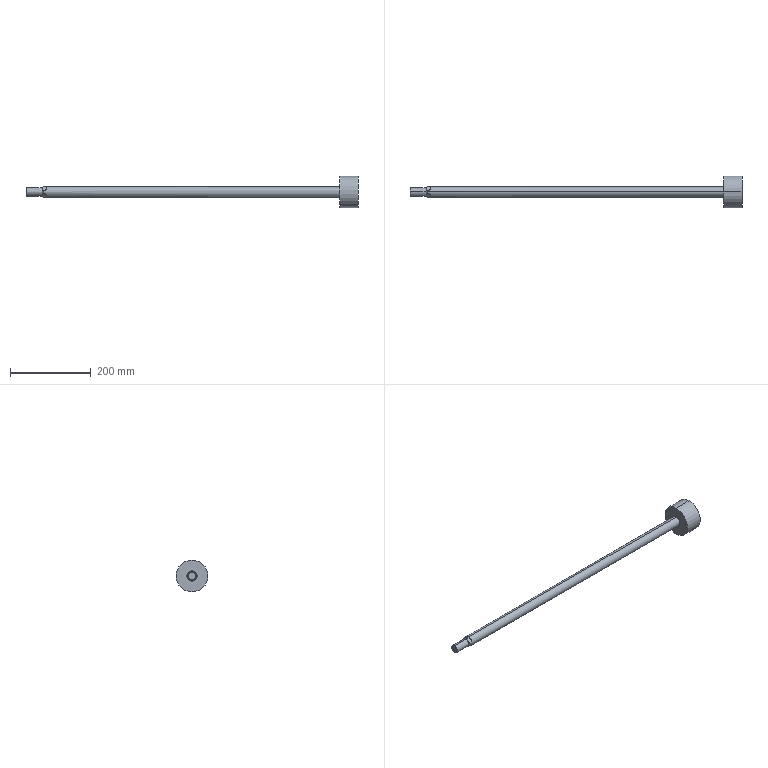Part | NX | features BREP 1 | 1 solid | 21 faces | box 822.5 x 78.6 x 78.6 mm | volume 592313 mm3 | plane 11 | cylinder 6 | cone 4 | commonest cylinder face diameters 20 x2 25 x2 78.6 x2
STEP:
#1=CARTESIAN_POINT('',(691.5,0.,12.5));
#2=VERTEX_POINT('',#1);
#3=CARTESIAN_POINT('',(691.5,0.,-12.5));
#4=VERTEX_POINT('',#3);
#5=CARTESIAN_POINT('',(691.5,0.,0.));
#6=DIRECTION('',(-1.,0.,0.));
#7=DIRECTION('',(0.,0.,1.));
#8=AXIS2_PLACEMENT_3D('',#5,#6,#7);
#9=CIRCLE('',#8,12.5);
#10=EDGE_CURVE('',#2,#4,#9,.T.);
#11=ORIENTED_EDGE('',*,*,#10,.T.);
#12=CARTESIAN_POINT('',(-43.5,0.,-12.5));
#13=VERTEX_POINT('',#12);
#14=CARTESIAN_POINT('',(736.5,0.,-12.5));
#15=DIRECTION('',(-1.,0.,0.));
#16=VECTOR('',#15,1000.);
#17=LINE('',#14,#16);
#18=EDGE_CURVE('',#13,#4,#17,.F.);
#19=ORIENTED_EDGE('',*,*,#18,.F.);
#20=CARTESIAN_POINT('',(-43.5,3.58,-11.976));
#21=VERTEX_POINT('',#20);
#22=CARTESIAN_POINT('',(-43.5,0.,0.));
#23=DIRECTION('',(1.,0.,0.));
#24=DIRECTION('',(0.,0.,1.));
#25=AXIS2_PLACEMENT_3D('',#22,#23,#24);
#26=CIRCLE('',#25,12.5);
#27=EDGE_CURVE('',#13,#21,#26,.T.);
#28=ORIENTED_EDGE('',*,*,#27,.T.);
#29=CARTESIAN_POINT('',(-37.1,3.58,-11.976));
#30=VERTEX_POINT('',#29);
#31=CARTESIAN_POINT('',(736.5,3.58,-11.976));
#32=DIRECTION('',(1.,0.,0.));
#33=VECTOR('',#32,1000.);
#34=LINE('',#31,#33);
#35=EDGE_CURVE('',#21,#30,#34,.T.);
#36=ORIENTED_EDGE('',*,*,#35,.T.);
#37=CARTESIAN_POINT('',(-37.1,11.976,-3.58));
#38=VERTEX_POINT('',#37);
#39=CARTESIAN_POINT('',(-37.1,3.58,-11.976));
#40=CARTESIAN_POINT('',(-35.057,7.702,-10.744));
#41=CARTESIAN_POINT('',(-35.057,10.744,-7.702));
#42=CARTESIAN_POINT('',(-37.1,11.976,-3.58));
#43=(BOUNDED_CURVE()B_SPLINE_CURVE(3,(#39,#40,#41,#42),.UNSPECIFIED.,.F.,.F.)B_SPLINE_CURVE_WITH_KNOTS((4,4),(2.647,3.637),.UNSPECIFIED.)CURVE()GEOMETRIC_REPRESENTATION_ITEM()RATIONAL_B_SPLINE_CURVE((1.,0.92,0.92,1.))REPRESENTATION_ITEM(''));
#44=EDGE_CURVE('',#30,#38,#43,.T.);
#45=ORIENTED_EDGE('',*,*,#44,.T.);
#46=CARTESIAN_POINT('',(-43.5,11.976,-3.58));
#47=VERTEX_POINT('',#46);
#48=CARTESIAN_POINT('',(736.5,11.976,-3.58));
#49=DIRECTION('',(-1.,0.,0.));
#50=VECTOR('',#49,1000.);
#51=LINE('',#48,#50);
#52=EDGE_CURVE('',#38,#47,#51,.T.);
#53=ORIENTED_EDGE('',*,*,#52,.T.);
#54=CARTESIAN_POINT('',(-43.5,11.976,3.58));
#55=VERTEX_POINT('',#54);
#56=CARTESIAN_POINT('',(-43.5,0.,0.));
#57=DIRECTION('',(1.,0.,0.));
#58=DIRECTION('',(0.,0.,1.));
#59=AXIS2_PLACEMENT_3D('',#56,#57,#58);
#60=CIRCLE('',#59,12.5);
#61=EDGE_CURVE('',#47,#55,#60,.T.);
#62=ORIENTED_EDGE('',*,*,#61,.T.);
#63=CARTESIAN_POINT('',(-37.1,11.976,3.58));
#64=VERTEX_POINT('',#63);
#65=CARTESIAN_POINT('',(736.5,11.976,3.58));
#66=DIRECTION('',(1.,0.,0.));
#67=VECTOR('',#66,1000.);
#68=LINE('',#65,#67);
#69=EDGE_CURVE('',#55,#64,#68,.T.);
#70=ORIENTED_EDGE('',*,*,#69,.T.);
#71=CARTESIAN_POINT('',(-37.1,3.58,11.976));
#72=VERTEX_POINT('',#71);
#73=CARTESIAN_POINT('',(-37.1,11.976,3.58));
#74=CARTESIAN_POINT('',(-35.057,10.744,7.702));
#75=CARTESIAN_POINT('',(-35.057,7.702,10.744));
#76=CARTESIAN_POINT('',(-37.1,3.58,11.976));
#77=(BOUNDED_CURVE()B_SPLINE_CURVE(3,(#73,#74,#75,#76),.UNSPECIFIED.,.F.,.F.)B_SPLINE_CURVE_WITH_KNOTS((4,4),(2.647,3.637),.UNSPECIFIED.)CURVE()GEOMETRIC_REPRESENTATION_ITEM()RATIONAL_B_SPLINE_CURVE((1.,0.92,0.92,1.))REPRESENTATION_ITEM(''));
#78=EDGE_CURVE('',#64,#72,#77,.T.);
#79=ORIENTED_EDGE('',*,*,#78,.T.);
#80=CARTESIAN_POINT('',(-43.5,3.58,11.976));
#81=VERTEX_POINT('',#80);
#82=CARTESIAN_POINT('',(736.5,3.58,11.976));
#83=DIRECTION('',(-1.,0.,0.));
#84=VECTOR('',#83,1000.);
#85=LINE('',#82,#84);
#86=EDGE_CURVE('',#72,#81,#85,.T.);
#87=ORIENTED_EDGE('',*,*,#86,.T.);
#88=CARTESIAN_POINT('',(-43.5,0.,12.5));
#89=VERTEX_POINT('',#88);
#90=CARTESIAN_POINT('',(-43.5,0.,0.));
#91=DIRECTION('',(1.,0.,0.));
#92=DIRECTION('',(0.,0.,1.));
#93=AXIS2_PLACEMENT_3D('',#90,#91,#92);
#94=CIRCLE('',#93,12.5);
#95=EDGE_CURVE('',#81,#89,#94,.T.);
#96=ORIENTED_EDGE('',*,*,#95,.T.);
#97=CARTESIAN_POINT('',(736.5,0.,12.5));
#98=DIRECTION('',(-1.,0.,0.));
#99=VECTOR('',#98,1000.);
#100=LINE('',#97,#99);
#101=EDGE_CURVE('',#89,#2,#100,.F.);
#102=ORIENTED_EDGE('',*,*,#101,.T.);
#103=EDGE_LOOP('',(#11,#19,#28,#36,#45,#53,#62,#70,#79,#87,#96,#102));
#104=FACE_BOUND('',#103,.T.);
#105=CARTESIAN_POINT('',(736.5,0.,0.));
#106=DIRECTION('',(-1.,0.,0.));
#107=DIRECTION('',(0.,0.,1.));
#108=AXIS2_PLACEMENT_3D('',#105,#106,#107);
#109=CYLINDRICAL_SURFACE('',#108,12.5);
#110=ADVANCED_FACE('',(#104),#109,.T.);
#111=CARTESIAN_POINT('',(-46.,0.,-10.));
#112=VERTEX_POINT('',#111);
#113=CARTESIAN_POINT('',(-46.,0.,10.));
#114=VERTEX_POINT('',#113);
#115=CARTESIAN_POINT('',(-46.,0.,0.));
#116=DIRECTION('',(1.,0.,0.));
#117=DIRECTION('',(0.,0.,-1.));
#118=AXIS2_PLACEMENT_3D('',#115,#116,#117);
#119=CIRCLE('',#118,10.);
#120=EDGE_CURVE('',#112,#114,#119,.T.);
#121=ORIENTED_EDGE('',*,*,#120,.T.);
#122=CARTESIAN_POINT('',(-43.5,0.,12.5));
#123=DIRECTION('',(0.7071,0.,0.7071));
#124=VECTOR('',#123,1000.);
#125=LINE('',#122,#124);
#126=EDGE_CURVE('',#114,#89,#125,.T.);
#127=ORIENTED_EDGE('',*,*,#126,.T.);
#128=ORIENTED_EDGE('',*,*,#95,.F.);
#129=CARTESIAN_POINT('',(-43.5,11.976,3.58));
#130=CARTESIAN_POINT('',(-43.979,11.263,4.294));
#131=CARTESIAN_POINT('',(-44.505,10.309,5.247));
#132=CARTESIAN_POINT('',(-44.937,8.824,6.732));
#133=CARTESIAN_POINT('',(-45.032,7.764,7.792));
#134=CARTESIAN_POINT('',(-44.933,6.711,8.845));
#135=CARTESIAN_POINT('',(-44.598,5.578,9.979));
#136=CARTESIAN_POINT('',(-44.158,4.637,10.919));
#137=CARTESIAN_POINT('',(-43.738,3.934,11.623));
#138=CARTESIAN_POINT('',(-43.5,3.58,11.976));
#139=B_SPLINE_CURVE_WITH_KNOTS('',3,(#129,#130,#131,#132,#133,#134,#135,#136,#137,#138),.UNSPECIFIED.,.F.,.F.,(4,1,1,1,1,1,1,4),(0.,0.25,0.375,0.5,0.625,0.75,0.875,1.),.UNSPECIFIED.);
#140=EDGE_CURVE('',#81,#55,#139,.F.);
#141=ORIENTED_EDGE('',*,*,#140,.T.);
#142=ORIENTED_EDGE('',*,*,#61,.F.);
#143=CARTESIAN_POINT('',(-43.5,3.58,-11.976));
#144=CARTESIAN_POINT('',(-43.979,4.294,-11.263));
#145=CARTESIAN_POINT('',(-44.505,5.247,-10.309));
#146=CARTESIAN_POINT('',(-44.937,6.732,-8.824));
#147=CARTESIAN_POINT('',(-45.032,7.792,-7.764));
#148=CARTESIAN_POINT('',(-44.933,8.845,-6.711));
#149=CARTESIAN_POINT('',(-44.598,9.979,-5.578));
#150=CARTESIAN_POINT('',(-44.158,10.919,-4.637));
#151=CARTESIAN_POINT('',(-43.738,11.623,-3.934));
#152=CARTESIAN_POINT('',(-43.5,11.976,-3.58));
#153=B_SPLINE_CURVE_WITH_KNOTS('',3,(#143,#144,#145,#146,#147,#148,#149,#150,#151,#152),.UNSPECIFIED.,.F.,.F.,(4,1,1,1,1,1,1,4),(0.,0.25,0.375,0.5,0.625,0.75,0.875,1.),.UNSPECIFIED.);
#154=EDGE_CURVE('',#47,#21,#153,.F.);
#155=ORIENTED_EDGE('',*,*,#154,.T.);
#156=ORIENTED_EDGE('',*,*,#27,.F.);
#157=CARTESIAN_POINT('',(-43.5,0.,-12.5));
#158=DIRECTION('',(0.7071,0.,-0.7071));
#159=VECTOR('',#158,1000.);
#160=LINE('',#157,#159);
#161=EDGE_CURVE('',#112,#13,#160,.T.);
#162=ORIENTED_EDGE('',*,*,#161,.F.);
#163=EDGE_LOOP('',(#121,#127,#128,#141,#142,#155,#156,#162));
#164=FACE_BOUND('',#163,.T.);
#165=CARTESIAN_POINT('',(-43.5,0.,0.));
#166=DIRECTION('',(1.,0.,0.));
#167=DIRECTION('',(0.,0.,-1.));
#168=AXIS2_PLACEMENT_3D('',#165,#166,#167);
#169=CONICAL_SURFACE('',#168,12.5,0.7854);
#170=ADVANCED_FACE('',(#164),#169,.T.);
#171=ORIENTED_EDGE('',*,*,#120,.F.);
#172=CARTESIAN_POINT('',(-85.08,0.,-10.));
#173=VERTEX_POINT('',#172);
#174=CARTESIAN_POINT('',(736.5,0.,-10.));
#175=DIRECTION('',(-1.,0.,0.));
#176=VECTOR('',#175,1000.);
#177=LINE('',#174,#176);
#178=EDGE_CURVE('',#173,#112,#177,.F.);
#179=ORIENTED_EDGE('',*,*,#178,.F.);
#180=CARTESIAN_POINT('',(-85.08,0.,10.));
#181=VERTEX_POINT('',#180);
#182=CARTESIAN_POINT('',(-85.08,0.,0.));
#183=DIRECTION('',(1.,0.,0.));
#184=DIRECTION('',(0.,0.,1.));
#185=AXIS2_PLACEMENT_3D('',#182,#183,#184);
#186=CIRCLE('',#185,10.);
#187=EDGE_CURVE('',#173,#181,#186,.T.);
#188=ORIENTED_EDGE('',*,*,#187,.T.);
#189=CARTESIAN_POINT('',(736.5,0.,10.));
#190=DIRECTION('',(-1.,0.,0.));
#191=VECTOR('',#190,1000.);
#192=LINE('',#189,#191);
#193=EDGE_CURVE('',#181,#114,#192,.F.);
#194=ORIENTED_EDGE('',*,*,#193,.T.);
#195=EDGE_LOOP('',(#171,#179,#188,#194));
#196=FACE_BOUND('',#195,.T.);
#197=CARTESIAN_POINT('',(736.5,0.,0.));
#198=DIRECTION('',(-1.,0.,0.));
#199=DIRECTION('',(0.,0.,1.));
#200=AXIS2_PLACEMENT_3D('',#197,#198,#199);
#201=CYLINDRICAL_SURFACE('',#200,10.);
#202=ADVANCED_FACE('',(#196),#201,.T.);
#203=CARTESIAN_POINT('',(736.5,0.,39.3));
#204=VERTEX_POINT('',#203);
#205=CARTESIAN_POINT('',(736.5,0.,-39.3));
#206=VERTEX_POINT('',#205);
#207=CARTESIAN_POINT('',(736.5,0.,0.));
#208=DIRECTION('',(-1.,0.,0.));
#209=DIRECTION('',(0.,0.,1.));
#210=AXIS2_PLACEMENT_3D('',#207,#208,#209);
#211=CIRCLE('',#210,39.3);
#212=EDGE_CURVE('',#204,#206,#211,.T.);
#213=ORIENTED_EDGE('',*,*,#212,.T.);
#214=CARTESIAN_POINT('',(691.5,0.,-39.3));
#215=VERTEX_POINT('',#214);
#216=CARTESIAN_POINT('',(736.5,0.,-39.3));
#217=DIRECTION('',(-1.,0.,0.));
#218=VECTOR('',#217,1000.);
#219=LINE('',#216,#218);
#220=EDGE_CURVE('',#215,#206,#219,.F.);
#221=ORIENTED_EDGE('',*,*,#220,.F.);
#222=CARTESIAN_POINT('',(691.5,0.,39.3));
#223=VERTEX_POINT('',#222);
#224=CARTESIAN_POINT('',(691.5,0.,0.));
#225=DIRECTION('',(1.,0.,0.));
#226=DIRECTION('',(0.,0.,1.));
#227=AXIS2_PLACEMENT_3D('',#224,#225,#226);
#228=CIRCLE('',#227,39.3);
#229=EDGE_CURVE('',#215,#223,#228,.T.);
#230=ORIENTED_EDGE('',*,*,#229,.T.);
#231=CARTESIAN_POINT('',(736.5,0.,39.3));
#232=DIRECTION('',(-1.,0.,0.));
#233=VECTOR('',#232,1000.);
#234=LINE('',#231,#233);
#235=EDGE_CURVE('',#223,#204,#234,.F.);
#236=ORIENTED_EDGE('',*,*,#235,.T.);
#237=EDGE_LOOP('',(#213,#221,#230,#236));
#238=FACE_BOUND('',#237,.T.);
#239=CARTESIAN_POINT('',(736.5,0.,0.));
#240=DIRECTION('',(-1.,0.,0.));
#241=DIRECTION('',(0.,0.,1.));
#242=AXIS2_PLACEMENT_3D('',#239,#240,#241);
#243=CYLINDRICAL_SURFACE('',#242,39.3);
#244=ADVANCED_FACE('',(#238),#243,.T.);
#245=CARTESIAN_POINT('',(-86.,0.,-9.08));
#246=VERTEX_POINT('',#245);
#247=CARTESIAN_POINT('',(-86.,0.,9.08));
#248=VERTEX_POINT('',#247);
#249=CARTESIAN_POINT('',(-86.,0.,0.));
#250=DIRECTION('',(1.,0.,0.));
#251=DIRECTION('',(0.,0.,-1.));
#252=AXIS2_PLACEMENT_3D('',#249,#250,#251);
#253=CIRCLE('',#252,9.08);
#254=EDGE_CURVE('',#246,#248,#253,.T.);
#255=ORIENTED_EDGE('',*,*,#254,.T.);
#256=CARTESIAN_POINT('',(-85.08,0.,10.));
#257=DIRECTION('',(0.7071,0.,0.7071));
#258=VECTOR('',#257,1000.);
#259=LINE('',#256,#258);
#260=EDGE_CURVE('',#248,#181,#259,.T.);
#261=ORIENTED_EDGE('',*,*,#260,.T.);
#262=ORIENTED_EDGE('',*,*,#187,.F.);
#263=CARTESIAN_POINT('',(-85.08,0.,-10.));
#264=DIRECTION('',(0.7071,0.,-0.7071));
#265=VECTOR('',#264,1000.);
#266=LINE('',#263,#265);
#267=EDGE_CURVE('',#246,#173,#266,.T.);
#268=ORIENTED_EDGE('',*,*,#267,.F.);
#269=EDGE_LOOP('',(#255,#261,#262,#268));
#270=FACE_BOUND('',#269,.T.);
#271=CARTESIAN_POINT('',(-85.08,0.,0.));
#272=DIRECTION('',(1.,0.,0.));
#273=DIRECTION('',(0.,0.,-1.));
#274=AXIS2_PLACEMENT_3D('',#271,#272,#273);
#275=CONICAL_SURFACE('',#274,10.,0.7854);
#276=ADVANCED_FACE('',(#270),#275,.T.);
#277=ORIENTED_EDGE('',*,*,#18,.T.);
#278=CARTESIAN_POINT('',(691.5,0.,0.));
#279=DIRECTION('',(-1.,0.,0.));
#280=DIRECTION('',(0.,0.,1.));
#281=AXIS2_PLACEMENT_3D('',#278,#279,#280);
#282=CIRCLE('',#281,12.5);
#283=EDGE_CURVE('',#4,#2,#282,.T.);
#284=ORIENTED_EDGE('',*,*,#283,.T.);
#285=ORIENTED_EDGE('',*,*,#101,.F.);
#286=CARTESIAN_POINT('',(-43.5,-3.58,11.976));
#287=VERTEX_POINT('',#286);
#288=CARTESIAN_POINT('',(-43.5,0.,0.));
#289=DIRECTION('',(1.,0.,0.));
#290=DIRECTION('',(0.,0.,1.));
#291=AXIS2_PLACEMENT_3D('',#288,#289,#290);
#292=CIRCLE('',#291,12.5);
#293=EDGE_CURVE('',#89,#287,#292,.T.);
#294=ORIENTED_EDGE('',*,*,#293,.T.);
#295=CARTESIAN_POINT('',(-37.1,-3.58,11.976));
#296=VERTEX_POINT('',#295);
#297=CARTESIAN_POINT('',(736.5,-3.58,11.976));
#298=DIRECTION('',(1.,0.,0.));
#299=VECTOR('',#298,1000.);
#300=LINE('',#297,#299);
#301=EDGE_CURVE('',#287,#296,#300,.T.);
#302=ORIENTED_EDGE('',*,*,#301,.T.);
#303=CARTESIAN_POINT('',(-37.1,-11.976,3.58));
#304=VERTEX_POINT('',#303);
#305=CARTESIAN_POINT('',(-37.1,-3.58,11.976));
#306=CARTESIAN_POINT('',(-35.057,-7.702,10.744));
#307=CARTESIAN_POINT('',(-35.057,-10.744,7.702));
#308=CARTESIAN_POINT('',(-37.1,-11.976,3.58));
#309=(BOUNDED_CURVE()B_SPLINE_CURVE(3,(#305,#306,#307,#308),.UNSPECIFIED.,.F.,.F.)B_SPLINE_CURVE_WITH_KNOTS((4,4),(2.647,3.637),.UNSPECIFIED.)CURVE()GEOMETRIC_REPRESENTATION_ITEM()RATIONAL_B_SPLINE_CURVE((1.,0.92,0.92,1.))REPRESENTATION_ITEM(''));
#310=EDGE_CURVE('',#296,#304,#309,.T.);
#311=ORIENTED_EDGE('',*,*,#310,.T.);
#312=CARTESIAN_POINT('',(-43.5,-11.976,3.58));
#313=VERTEX_POINT('',#312);
#314=CARTESIAN_POINT('',(736.5,-11.976,3.58));
#315=DIRECTION('',(-1.,0.,0.));
#316=VECTOR('',#315,1000.);
#317=LINE('',#314,#316);
#318=EDGE_CURVE('',#304,#313,#317,.T.);
#319=ORIENTED_EDGE('',*,*,#318,.T.);
#320=CARTESIAN_POINT('',(-43.5,-11.976,-3.58));
#321=VERTEX_POINT('',#320);
#322=CARTESIAN_POINT('',(-43.5,0.,0.));
#323=DIRECTION('',(1.,0.,0.));
#324=DIRECTION('',(0.,0.,1.));
#325=AXIS2_PLACEMENT_3D('',#322,#323,#324);
#326=CIRCLE('',#325,12.5);
#327=EDGE_CURVE('',#313,#321,#326,.T.);
#328=ORIENTED_EDGE('',*,*,#327,.T.);
#329=CARTESIAN_POINT('',(-37.1,-11.976,-3.58));
#330=VERTEX_POINT('',#329);
#331=CARTESIAN_POINT('',(736.5,-11.976,-3.58));
#332=DIRECTION('',(1.,0.,0.));
#333=VECTOR('',#332,1000.);
#334=LINE('',#331,#333);
#335=EDGE_CURVE('',#321,#330,#334,.T.);
#336=ORIENTED_EDGE('',*,*,#335,.T.);
#337=CARTESIAN_POINT('',(-37.1,-3.58,-11.976));
#338=VERTEX_POINT('',#337);
#339=CARTESIAN_POINT('',(-37.1,-11.976,-3.58));
#340=CARTESIAN_POINT('',(-35.057,-10.744,-7.702));
#341=CARTESIAN_POINT('',(-35.057,-7.702,-10.744));
#342=CARTESIAN_POINT('',(-37.1,-3.58,-11.976));
#343=(BOUNDED_CURVE()B_SPLINE_CURVE(3,(#339,#340,#341,#342),.UNSPECIFIED.,.F.,.F.)B_SPLINE_CURVE_WITH_KNOTS((4,4),(2.647,3.637),.UNSPECIFIED.)CURVE()GEOMETRIC_REPRESENTATION_ITEM()RATIONAL_B_SPLINE_CURVE((1.,0.92,0.92,1.))REPRESENTATION_ITEM(''));
#344=EDGE_CURVE('',#330,#338,#343,.T.);
#345=ORIENTED_EDGE('',*,*,#344,.T.);
#346=CARTESIAN_POINT('',(-43.5,-3.58,-11.976));
#347=VERTEX_POINT('',#346);
#348=CARTESIAN_POINT('',(736.5,-3.58,-11.976));
#349=DIRECTION('',(-1.,0.,0.));
#350=VECTOR('',#349,1000.);
#351=LINE('',#348,#350);
#352=EDGE_CURVE('',#338,#347,#351,.T.);
#353=ORIENTED_EDGE('',*,*,#352,.T.);
#354=CARTESIAN_POINT('',(-43.5,0.,0.));
#355=DIRECTION('',(1.,0.,0.));
#356=DIRECTION('',(0.,0.,1.));
#357=AXIS2_PLACEMENT_3D('',#354,#355,#356);
#358=CIRCLE('',#357,12.5);
#359=EDGE_CURVE('',#347,#13,#358,.T.);
#360=ORIENTED_EDGE('',*,*,#359,.T.);
#361=EDGE_LOOP('',(#277,#284,#285,#294,#302,#311,#319,#328,#336,#345,#353,#360));
#362=FACE_BOUND('',#361,.T.);
#363=CARTESIAN_POINT('',(736.5,0.,0.));
#364=DIRECTION('',(-1.,0.,0.));
#365=DIRECTION('',(0.,0.,1.));
#366=AXIS2_PLACEMENT_3D('',#363,#364,#365);
#367=CYLINDRICAL_SURFACE('',#366,12.5);
#368=ADVANCED_FACE('',(#362),#367,.T.);
#369=ORIENTED_EDGE('',*,*,#344,.F.);
#370=CARTESIAN_POINT('',(-37.1,-11.976,-3.58));
#371=DIRECTION('',(0.,0.7071,-0.7071));
#372=VECTOR('',#371,1000.);
#373=LINE('',#370,#372);
#374=EDGE_CURVE('',#330,#338,#373,.T.);
#375=ORIENTED_EDGE('',*,*,#374,.T.);
#376=EDGE_LOOP('',(#369,#375));
#377=FACE_BOUND('',#376,.T.);
#378=CARTESIAN_POINT('',(-35.6,-16.617,-1.061));
#379=DIRECTION('',(-0.7071,-0.5,-0.5));
#380=DIRECTION('',(-0.5774,0.,0.8165));
#381=AXIS2_PLACEMENT_3D('',#378,#379,#380);
#382=PLANE('',#381);
#383=ADVANCED_FACE('',(#377),#382,.T.);
#384=ORIENTED_EDGE('',*,*,#335,.F.);
#385=CARTESIAN_POINT('',(-43.5,-11.976,-3.58));
#386=CARTESIAN_POINT('',(-43.737,-11.623,-3.933));
#387=CARTESIAN_POINT('',(-44.158,-10.92,-4.636));
#388=CARTESIAN_POINT('',(-44.598,-9.978,-5.578));
#389=CARTESIAN_POINT('',(-44.933,-8.846,-6.71));
#390=CARTESIAN_POINT('',(-45.032,-7.791,-7.766));
#391=CARTESIAN_POINT('',(-44.938,-6.736,-8.82));
#392=CARTESIAN_POINT('',(-44.61,-5.608,-9.949));
#393=CARTESIAN_POINT('',(-44.166,-4.65,-10.906));
#394=CARTESIAN_POINT('',(-43.741,-3.938,-11.618));
#395=CARTESIAN_POINT('',(-43.5,-3.58,-11.976));
#396=B_SPLINE_CURVE_WITH_KNOTS('',3,(#385,#386,#387,#388,#389,#390,#391,#392,#393,#394,#395),.UNSPECIFIED.,.F.,.F.,(4,1,1,1,1,1,1,1,4),(0.,0.125,0.25,0.375,0.5,0.625,0.75,0.875,1.),.UNSPECIFIED.);
#397=EDGE_CURVE('',#321,#347,#396,.T.);
#398=ORIENTED_EDGE('',*,*,#397,.T.);
#399=ORIENTED_EDGE('',*,*,#352,.F.);
#400=ORIENTED_EDGE('',*,*,#374,.F.);
#401=EDGE_LOOP('',(#384,#398,#399,#400));
#402=FACE_BOUND('',#401,.T.);
#403=CARTESIAN_POINT('',(-37.1,-15.556,0.));
#404=DIRECTION('',(0.,-0.7071,-0.7071));
#405=DIRECTION('',(0.,0.7071,-0.7071));
#406=AXIS2_PLACEMENT_3D('',#403,#404,#405);
#407=PLANE('',#406);
#408=ADVANCED_FACE('',(#402),#407,.T.);
#409=ORIENTED_EDGE('',*,*,#126,.F.);
#410=CARTESIAN_POINT('',(-46.,0.,0.));
#411=DIRECTION('',(1.,0.,0.));
#412=DIRECTION('',(0.,0.,-1.));
#413=AXIS2_PLACEMENT_3D('',#410,#411,#412);
#414=CIRCLE('',#413,10.);
#415=EDGE_CURVE('',#114,#112,#414,.T.);
#416=ORIENTED_EDGE('',*,*,#415,.T.);
#417=ORIENTED_EDGE('',*,*,#161,.T.);
#418=ORIENTED_EDGE('',*,*,#359,.F.);
#419=ORIENTED_EDGE('',*,*,#397,.F.);
#420=ORIENTED_EDGE('',*,*,#327,.F.);
#421=CARTESIAN_POINT('',(-43.5,-3.58,11.976));
#422=CARTESIAN_POINT('',(-43.979,-4.294,11.263));
#423=CARTESIAN_POINT('',(-44.505,-5.247,10.309));
#424=CARTESIAN_POINT('',(-44.937,-6.732,8.824));
#425=CARTESIAN_POINT('',(-45.032,-7.792,7.764));
#426=CARTESIAN_POINT('',(-44.933,-8.845,6.711));
#427=CARTESIAN_POINT('',(-44.598,-9.979,5.578));
#428=CARTESIAN_POINT('',(-44.158,-10.919,4.637));
#429=CARTESIAN_POINT('',(-43.738,-11.623,3.934));
#430=CARTESIAN_POINT('',(-43.5,-11.976,3.58));
#431=B_SPLINE_CURVE_WITH_KNOTS('',3,(#421,#422,#423,#424,#425,#426,#427,#428,#429,#430),.UNSPECIFIED.,.F.,.F.,(4,1,1,1,1,1,1,4),(0.,0.25,0.375,0.5,0.625,0.75,0.875,1.),.UNSPECIFIED.);
#432=EDGE_CURVE('',#313,#287,#431,.F.);
#433=ORIENTED_EDGE('',*,*,#432,.T.);
#434=ORIENTED_EDGE('',*,*,#293,.F.);
#435=EDGE_LOOP('',(#409,#416,#417,#418,#419,#420,#433,#434));
#436=FACE_BOUND('',#435,.T.);
#437=CARTESIAN_POINT('',(-43.5,0.,0.));
#438=DIRECTION('',(1.,0.,0.));
#439=DIRECTION('',(0.,0.,-1.));
#440=AXIS2_PLACEMENT_3D('',#437,#438,#439);
#441=CONICAL_SURFACE('',#440,12.5,0.7854);
#442=ADVANCED_FACE('',(#436),#441,.T.);
#443=ORIENTED_EDGE('',*,*,#301,.F.);
#444=ORIENTED_EDGE('',*,*,#432,.F.);
#445=ORIENTED_EDGE('',*,*,#318,.F.);
#446=CARTESIAN_POINT('',(-37.1,0.,15.556));
#447=DIRECTION('',(0.,0.7071,0.7071));
#448=VECTOR('',#447,1000.);
#449=LINE('',#446,#448);
#450=EDGE_CURVE('',#304,#296,#449,.T.);
#451=ORIENTED_EDGE('',*,*,#450,.T.);
#452=EDGE_LOOP('',(#443,#444,#445,#451));
#453=FACE_BOUND('',#452,.T.);
#454=CARTESIAN_POINT('',(-37.1,0.,15.556));
#455=DIRECTION('',(0.,-0.7071,0.7071));
#456=DIRECTION('',(-1.,0.,0.));
#457=AXIS2_PLACEMENT_3D('',#454,#455,#456);
#458=PLANE('',#457);
#459=ADVANCED_FACE('',(#453),#458,.T.);
#460=ORIENTED_EDGE('',*,*,#310,.F.);
#461=ORIENTED_EDGE('',*,*,#450,.F.);
#462=EDGE_LOOP('',(#460,#461));
#463=FACE_BOUND('',#462,.T.);
#464=CARTESIAN_POINT('',(-35.6,-1.061,16.617));
#465=DIRECTION('',(-0.7071,-0.5,0.5));
#466=DIRECTION('',(-0.5774,0.8165,0.));
#467=AXIS2_PLACEMENT_3D('',#464,#465,#466);
#468=PLANE('',#467);
#469=ADVANCED_FACE('',(#463),#468,.T.);
#470=ORIENTED_EDGE('',*,*,#69,.F.);
#471=ORIENTED_EDGE('',*,*,#140,.F.);
#472=ORIENTED_EDGE('',*,*,#86,.F.);
#473=CARTESIAN_POINT('',(-37.1,0.,15.556));
#474=DIRECTION('',(0.,0.7071,-0.7071));
#475=VECTOR('',#474,1000.);
#476=LINE('',#473,#475);
#477=EDGE_CURVE('',#72,#64,#476,.T.);
#478=ORIENTED_EDGE('',*,*,#477,.T.);
#479=EDGE_LOOP('',(#470,#471,#472,#478));
#480=FACE_BOUND('',#479,.T.);
#481=CARTESIAN_POINT('',(-89.3,0.,15.556));
#482=DIRECTION('',(0.,0.7071,0.7071));
#483=DIRECTION('',(1.,0.,0.));
#484=AXIS2_PLACEMENT_3D('',#481,#482,#483);
#485=PLANE('',#484);
#486=ADVANCED_FACE('',(#480),#485,.T.);
#487=ORIENTED_EDGE('',*,*,#78,.F.);
#488=ORIENTED_EDGE('',*,*,#477,.F.);
#489=EDGE_LOOP('',(#487,#488));
#490=FACE_BOUND('',#489,.T.);
#491=CARTESIAN_POINT('',(-37.1,0.,15.556));
#492=DIRECTION('',(-0.7071,0.5,0.5));
#493=DIRECTION('',(0.5774,0.,0.8165));
#494=AXIS2_PLACEMENT_3D('',#491,#492,#493);
#495=PLANE('',#494);
#496=ADVANCED_FACE('',(#490),#495,.T.);
#497=ORIENTED_EDGE('',*,*,#35,.F.);
#498=ORIENTED_EDGE('',*,*,#154,.F.);
#499=ORIENTED_EDGE('',*,*,#52,.F.);
#500=CARTESIAN_POINT('',(-37.1,15.556,0.));
#501=DIRECTION('',(0.,-0.7071,-0.7071));
#502=VECTOR('',#501,1000.);
#503=LINE('',#500,#502);
#504=EDGE_CURVE('',#38,#30,#503,.T.);
#505=ORIENTED_EDGE('',*,*,#504,.T.);
#506=EDGE_LOOP('',(#497,#498,#499,#505));
#507=FACE_BOUND('',#506,.T.);
#508=CARTESIAN_POINT('',(-89.3,15.556,0.));
#509=DIRECTION('',(0.,0.7071,-0.7071));
#510=DIRECTION('',(-1.,0.,0.));
#511=AXIS2_PLACEMENT_3D('',#508,#509,#510);
#512=PLANE('',#511);
#513=ADVANCED_FACE('',(#507),#512,.T.);
#514=ORIENTED_EDGE('',*,*,#44,.F.);
#515=ORIENTED_EDGE('',*,*,#504,.F.);
#516=EDGE_LOOP('',(#514,#515));
#517=FACE_BOUND('',#516,.T.);
#518=CARTESIAN_POINT('',(-37.1,15.556,0.));
#519=DIRECTION('',(-0.7071,0.5,-0.5));
#520=DIRECTION('',(-0.5774,0.,0.8165));
#521=AXIS2_PLACEMENT_3D('',#518,#519,#520);
#522=PLANE('',#521);
#523=ADVANCED_FACE('',(#517),#522,.T.);
#524=CARTESIAN_POINT('',(691.5,0.,0.));
#525=DIRECTION('',(1.,0.,0.));
#526=DIRECTION('',(0.,0.,1.));
#527=AXIS2_PLACEMENT_3D('',#524,#525,#526);
#528=CIRCLE('',#527,39.3);
#529=EDGE_CURVE('',#223,#215,#528,.T.);
#530=ORIENTED_EDGE('',*,*,#529,.F.);
#531=ORIENTED_EDGE('',*,*,#229,.F.);
#532=EDGE_LOOP('',(#530,#531));
#533=FACE_BOUND('',#532,.T.);
#534=ORIENTED_EDGE('',*,*,#10,.F.);
#535=ORIENTED_EDGE('',*,*,#283,.F.);
#536=EDGE_LOOP('',(#534,#535));
#537=FACE_BOUND('',#536,.T.);
#538=CARTESIAN_POINT('',(691.5,12.5,0.));
#539=DIRECTION('',(1.,0.,0.));
#540=DIRECTION('',(0.,1.,0.));
#541=AXIS2_PLACEMENT_3D('',#538,#539,#540);
#542=PLANE('',#541);
#543=ADVANCED_FACE('',(#533,#537),#542,.F.);
#544=ORIENTED_EDGE('',*,*,#178,.T.);
#545=ORIENTED_EDGE('',*,*,#415,.F.);
#546=ORIENTED_EDGE('',*,*,#193,.F.);
#547=CARTESIAN_POINT('',(-85.08,0.,0.));
#548=DIRECTION('',(1.,0.,0.));
#549=DIRECTION('',(0.,0.,1.));
#550=AXIS2_PLACEMENT_3D('',#547,#548,#549);
#551=CIRCLE('',#550,10.);
#552=EDGE_CURVE('',#181,#173,#551,.T.);
#553=ORIENTED_EDGE('',*,*,#552,.T.);
#554=EDGE_LOOP('',(#544,#545,#546,#553));
#555=FACE_BOUND('',#554,.T.);
#556=CARTESIAN_POINT('',(736.5,0.,0.));
#557=DIRECTION('',(-1.,0.,0.));
#558=DIRECTION('',(0.,0.,1.));
#559=AXIS2_PLACEMENT_3D('',#556,#557,#558);
#560=CYLINDRICAL_SURFACE('',#559,10.);
#561=ADVANCED_FACE('',(#555),#560,.T.);
#562=ORIENTED_EDGE('',*,*,#220,.T.);
#563=CARTESIAN_POINT('',(736.5,0.,0.));
#564=DIRECTION('',(-1.,0.,0.));
#565=DIRECTION('',(0.,0.,1.));
#566=AXIS2_PLACEMENT_3D('',#563,#564,#565);
#567=CIRCLE('',#566,39.3);
#568=EDGE_CURVE('',#206,#204,#567,.T.);
#569=ORIENTED_EDGE('',*,*,#568,.T.);
#570=ORIENTED_EDGE('',*,*,#235,.F.);
#571=ORIENTED_EDGE('',*,*,#529,.T.);
#572=EDGE_LOOP('',(#562,#569,#570,#571));
#573=FACE_BOUND('',#572,.T.);
#574=CARTESIAN_POINT('',(736.5,0.,0.));
#575=DIRECTION('',(-1.,0.,0.));
#576=DIRECTION('',(0.,0.,1.));
#577=AXIS2_PLACEMENT_3D('',#574,#575,#576);
#578=CYLINDRICAL_SURFACE('',#577,39.3);
#579=ADVANCED_FACE('',(#573),#578,.T.);
#580=ORIENTED_EDGE('',*,*,#260,.F.);
#581=CARTESIAN_POINT('',(-86.,0.,0.));
#582=DIRECTION('',(1.,0.,0.));
#583=DIRECTION('',(0.,0.,-1.));
#584=AXIS2_PLACEMENT_3D('',#581,#582,#583);
#585=CIRCLE('',#584,9.08);
#586=EDGE_CURVE('',#248,#246,#585,.T.);
#587=ORIENTED_EDGE('',*,*,#586,.T.);
#588=ORIENTED_EDGE('',*,*,#267,.T.);
#589=ORIENTED_EDGE('',*,*,#552,.F.);
#590=EDGE_LOOP('',(#580,#587,#588,#589));
#591=FACE_BOUND('',#590,.T.);
#592=CARTESIAN_POINT('',(-85.08,0.,0.));
#593=DIRECTION('',(1.,0.,0.));
#594=DIRECTION('',(0.,0.,-1.));
#595=AXIS2_PLACEMENT_3D('',#592,#593,#594);
#596=CONICAL_SURFACE('',#595,10.,0.7854);
#597=ADVANCED_FACE('',(#591),#596,.T.);
#598=ORIENTED_EDGE('',*,*,#212,.F.);
#599=ORIENTED_EDGE('',*,*,#568,.F.);
#600=EDGE_LOOP('',(#598,#599));
#601=FACE_BOUND('',#600,.T.);
#602=CARTESIAN_POINT('',(736.5,39.3,0.));
#603=DIRECTION('',(-1.,0.,0.));
#604=DIRECTION('',(0.,0.,1.));
#605=AXIS2_PLACEMENT_3D('',#602,#603,#604);
#606=PLANE('',#605);
#607=ADVANCED_FACE('',(#601),#606,.F.);
#608=ORIENTED_EDGE('',*,*,#254,.F.);
#609=ORIENTED_EDGE('',*,*,#586,.F.);
#610=EDGE_LOOP('',(#608,#609));
#611=FACE_BOUND('',#610,.T.);
#612=CARTESIAN_POINT('',(-86.,0.,0.));
#613=DIRECTION('',(1.,0.,0.));
#614=DIRECTION('',(0.,1.,0.));
#615=AXIS2_PLACEMENT_3D('',#612,#613,#614);
#616=PLANE('',#615);
#617=ADVANCED_FACE('',(#611),#616,.F.);
#618=CLOSED_SHELL('',(#110,#170,#202,#244,#276,#368,#383,#408,#442,#459,#469,#486,#496,#513,#523,#543,#561,#579,#597,#607,#617));
#619=MANIFOLD_SOLID_BREP('',#618);
#620=(LENGTH_UNIT()NAMED_UNIT(*)SI_UNIT(.MILLI.,.METRE.));
#621=UNCERTAINTY_MEASURE_WITH_UNIT(LENGTH_MEASURE(0.0508),#620,'','');
#622=(NAMED_UNIT(*)PLANE_ANGLE_UNIT()SI_UNIT($,.RADIAN.));
#623=(NAMED_UNIT(*)SI_UNIT($,.STERADIAN.)SOLID_ANGLE_UNIT());
#624=(GEOMETRIC_REPRESENTATION_CONTEXT(3)GLOBAL_UNCERTAINTY_ASSIGNED_CONTEXT((#621))GLOBAL_UNIT_ASSIGNED_CONTEXT((#620,#622,#623))REPRESENTATION_CONTEXT('',''));
#625=ADVANCED_BREP_SHAPE_REPRESENTATION('',(#619),#624);